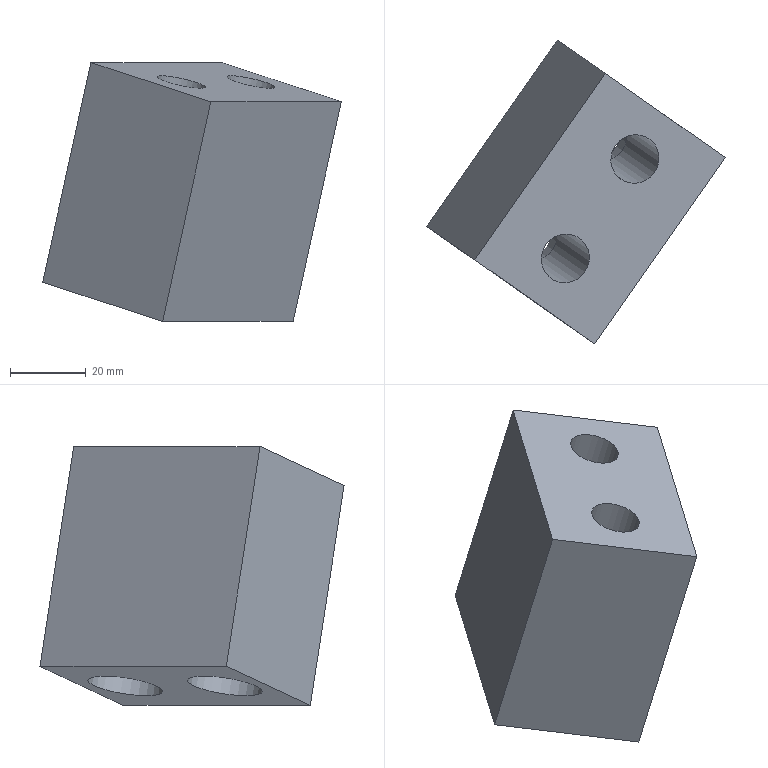Part | NX | features solid 2 | 1 solid | 12 faces | box 78.785 x 80.218 x 68.308 mm | volume 120815 mm3 | plane 8 | cylinder 4 | commonest cylinder face diameters 13 x2 20 x2
STEP:
#1=CARTESIAN_POINT('',(27.002,617.117,-490.837));
#2=VERTEX_POINT('',#1);
#3=CARTESIAN_POINT('',(21.858,620.718,-489.155));
#4=DIRECTION('',(-0.212,0.1485,-0.9659));
#5=DIRECTION('',(0.7912,-0.554,-0.2588));
#6=AXIS2_PLACEMENT_3D('',#3,#4,#5);
#7=CIRCLE('',#6,6.5);
#8=EDGE_CURVE('',#2,#2,#7,.F.);
#9=ORIENTED_EDGE('',*,*,#8,.F.);
#10=EDGE_LOOP('',(#9));
#11=FACE_BOUND('',#10,.T.);
#12=CARTESIAN_POINT('',(8.647,590.904,-490.837));
#13=VERTEX_POINT('',#12);
#14=CARTESIAN_POINT('',(3.504,594.505,-489.155));
#15=DIRECTION('',(-0.212,0.1485,-0.9659));
#16=DIRECTION('',(0.7912,-0.554,-0.2588));
#17=AXIS2_PLACEMENT_3D('',#14,#15,#16);
#18=CIRCLE('',#17,6.5);
#19=EDGE_CURVE('',#13,#13,#18,.F.);
#20=ORIENTED_EDGE('',*,*,#19,.F.);
#21=EDGE_LOOP('',(#20));
#22=FACE_BOUND('',#21,.T.);
#23=CARTESIAN_POINT('',(11.299,571.956,-494.331));
#24=VERTEX_POINT('',#23);
#25=CARTESIAN_POINT('',(-20.351,594.118,-483.978));
#26=VERTEX_POINT('',#25);
#27=CARTESIAN_POINT('',(11.299,571.956,-494.331));
#28=DIRECTION('',(0.7912,-0.554,-0.2588));
#29=VECTOR('',#28,1000.);
#30=LINE('',#27,#29);
#31=EDGE_CURVE('',#24,#26,#30,.F.);
#32=ORIENTED_EDGE('',*,*,#31,.F.);
#33=CARTESIAN_POINT('',(45.713,621.106,-494.331));
#34=VERTEX_POINT('',#33);
#35=CARTESIAN_POINT('',(45.713,621.106,-494.331));
#36=DIRECTION('',(-0.5736,-0.8192,0.));
#37=VECTOR('',#36,1000.);
#38=LINE('',#35,#37);
#39=EDGE_CURVE('',#34,#24,#38,.T.);
#40=ORIENTED_EDGE('',*,*,#39,.F.);
#41=CARTESIAN_POINT('',(14.064,643.267,-483.978));
#42=VERTEX_POINT('',#41);
#43=CARTESIAN_POINT('',(45.713,621.106,-494.331));
#44=DIRECTION('',(0.7912,-0.554,-0.2588));
#45=VECTOR('',#44,1000.);
#46=LINE('',#43,#45);
#47=EDGE_CURVE('',#34,#42,#46,.F.);
#48=ORIENTED_EDGE('',*,*,#47,.T.);
#49=CARTESIAN_POINT('',(14.064,643.267,-483.978));
#50=DIRECTION('',(-0.5736,-0.8192,0.));
#51=VECTOR('',#50,1000.);
#52=LINE('',#49,#51);
#53=EDGE_CURVE('',#42,#26,#52,.T.);
#54=ORIENTED_EDGE('',*,*,#53,.T.);
#55=EDGE_LOOP('',(#32,#40,#48,#54));
#56=FACE_BOUND('',#55,.T.);
#57=CARTESIAN_POINT('',(45.713,621.106,-494.331));
#58=DIRECTION('',(0.212,-0.1485,0.9659));
#59=DIRECTION('',(-0.5736,-0.8192,0.));
#60=AXIS2_PLACEMENT_3D('',#57,#58,#59);
#61=PLANE('',#60);
#62=ADVANCED_FACE('',(#11,#22,#56),#61,.T.);
#63=ORIENTED_EDGE('',*,*,#47,.F.);
#64=CARTESIAN_POINT('',(32.993,630.013,-552.287));
#65=VERTEX_POINT('',#64);
#66=CARTESIAN_POINT('',(45.713,621.106,-494.331));
#67=DIRECTION('',(-0.212,0.1485,-0.9659));
#68=VECTOR('',#67,1000.);
#69=LINE('',#66,#68);
#70=EDGE_CURVE('',#34,#65,#69,.T.);
#71=ORIENTED_EDGE('',*,*,#70,.T.);
#72=CARTESIAN_POINT('',(1.343,652.174,-541.934));
#73=VERTEX_POINT('',#72);
#74=CARTESIAN_POINT('',(32.993,630.013,-552.287));
#75=DIRECTION('',(-0.7912,0.554,0.2588));
#76=VECTOR('',#75,1000.);
#77=LINE('',#74,#76);
#78=EDGE_CURVE('',#65,#73,#77,.T.);
#79=ORIENTED_EDGE('',*,*,#78,.T.);
#80=CARTESIAN_POINT('',(14.064,643.267,-483.978));
#81=DIRECTION('',(0.212,-0.1485,0.9659));
#82=VECTOR('',#81,1000.);
#83=LINE('',#80,#82);
#84=EDGE_CURVE('',#42,#73,#83,.F.);
#85=ORIENTED_EDGE('',*,*,#84,.F.);
#86=EDGE_LOOP('',(#63,#71,#79,#85));
#87=FACE_BOUND('',#86,.T.);
#88=CARTESIAN_POINT('',(45.713,621.106,-494.331));
#89=DIRECTION('',(-0.5736,-0.8192,0.));
#90=DIRECTION('',(-0.212,0.1485,-0.9659));
#91=AXIS2_PLACEMENT_3D('',#88,#89,#90);
#92=PLANE('',#91);
#93=ADVANCED_FACE('',(#87),#92,.F.);
#94=CARTESIAN_POINT('',(17.05,624.085,-549.698));
#95=VERTEX_POINT('',#94);
#96=CARTESIAN_POINT('',(9.138,629.625,-547.11));
#97=DIRECTION('',(-0.212,0.1485,-0.9659));
#98=DIRECTION('',(0.7912,-0.554,-0.2588));
#99=AXIS2_PLACEMENT_3D('',#96,#97,#98);
#100=CIRCLE('',#99,10.);
#101=EDGE_CURVE('',#95,#95,#100,.T.);
#102=ORIENTED_EDGE('',*,*,#101,.F.);
#103=EDGE_LOOP('',(#102));
#104=FACE_BOUND('',#103,.T.);
#105=CARTESIAN_POINT('',(-1.304,597.872,-549.698));
#106=VERTEX_POINT('',#105);
#107=CARTESIAN_POINT('',(-9.217,603.412,-547.11));
#108=DIRECTION('',(-0.212,0.1485,-0.9659));
#109=DIRECTION('',(0.7912,-0.554,-0.2588));
#110=AXIS2_PLACEMENT_3D('',#107,#108,#109);
#111=CIRCLE('',#110,10.);
#112=EDGE_CURVE('',#106,#106,#111,.T.);
#113=ORIENTED_EDGE('',*,*,#112,.F.);
#114=EDGE_LOOP('',(#113));
#115=FACE_BOUND('',#114,.T.);
#116=ORIENTED_EDGE('',*,*,#78,.F.);
#117=CARTESIAN_POINT('',(-1.422,580.864,-552.287));
#118=VERTEX_POINT('',#117);
#119=CARTESIAN_POINT('',(32.993,630.013,-552.287));
#120=DIRECTION('',(-0.5736,-0.8192,0.));
#121=VECTOR('',#120,1000.);
#122=LINE('',#119,#121);
#123=EDGE_CURVE('',#65,#118,#122,.T.);
#124=ORIENTED_EDGE('',*,*,#123,.T.);
#125=CARTESIAN_POINT('',(-33.072,603.025,-541.934));
#126=VERTEX_POINT('',#125);
#127=CARTESIAN_POINT('',(-1.422,580.864,-552.287));
#128=DIRECTION('',(0.7912,-0.554,-0.2588));
#129=VECTOR('',#128,1000.);
#130=LINE('',#127,#129);
#131=EDGE_CURVE('',#118,#126,#130,.F.);
#132=ORIENTED_EDGE('',*,*,#131,.T.);
#133=CARTESIAN_POINT('',(1.343,652.174,-541.934));
#134=DIRECTION('',(-0.5736,-0.8192,0.));
#135=VECTOR('',#134,1000.);
#136=LINE('',#133,#135);
#137=EDGE_CURVE('',#73,#126,#136,.T.);
#138=ORIENTED_EDGE('',*,*,#137,.F.);
#139=EDGE_LOOP('',(#116,#124,#132,#138));
#140=FACE_BOUND('',#139,.T.);
#141=CARTESIAN_POINT('',(32.993,630.013,-552.287));
#142=DIRECTION('',(0.212,-0.1485,0.9659));
#143=DIRECTION('',(-0.5736,-0.8192,0.));
#144=AXIS2_PLACEMENT_3D('',#141,#142,#143);
#145=PLANE('',#144);
#146=ADVANCED_FACE('',(#104,#115,#140),#145,.F.);
#147=CARTESIAN_POINT('',(11.299,571.956,-494.331));
#148=DIRECTION('',(-0.212,0.1485,-0.9659));
#149=VECTOR('',#148,1000.);
#150=LINE('',#147,#149);
#151=EDGE_CURVE('',#24,#118,#150,.T.);
#152=ORIENTED_EDGE('',*,*,#151,.F.);
#153=ORIENTED_EDGE('',*,*,#31,.T.);
#154=CARTESIAN_POINT('',(-20.351,594.118,-483.978));
#155=DIRECTION('',(0.212,-0.1485,0.9659));
#156=VECTOR('',#155,1000.);
#157=LINE('',#154,#156);
#158=EDGE_CURVE('',#26,#126,#157,.F.);
#159=ORIENTED_EDGE('',*,*,#158,.T.);
#160=ORIENTED_EDGE('',*,*,#131,.F.);
#161=EDGE_LOOP('',(#152,#153,#159,#160));
#162=FACE_BOUND('',#161,.T.);
#163=CARTESIAN_POINT('',(11.299,571.956,-494.331));
#164=DIRECTION('',(-0.5736,-0.8192,0.));
#165=DIRECTION('',(-0.212,0.1485,-0.9659));
#166=AXIS2_PLACEMENT_3D('',#163,#164,#165);
#167=PLANE('',#166);
#168=ADVANCED_FACE('',(#162),#167,.T.);
#169=ORIENTED_EDGE('',*,*,#137,.T.);
#170=ORIENTED_EDGE('',*,*,#158,.F.);
#171=ORIENTED_EDGE('',*,*,#53,.F.);
#172=ORIENTED_EDGE('',*,*,#84,.T.);
#173=EDGE_LOOP('',(#169,#170,#171,#172));
#174=FACE_BOUND('',#173,.T.);
#175=CARTESIAN_POINT('',(14.064,643.267,-483.978));
#176=DIRECTION('',(-0.7912,0.554,0.2588));
#177=DIRECTION('',(0.212,-0.1485,0.9659));
#178=AXIS2_PLACEMENT_3D('',#175,#176,#177);
#179=PLANE('',#178);
#180=ADVANCED_FACE('',(#174),#179,.T.);
#181=ORIENTED_EDGE('',*,*,#123,.F.);
#182=ORIENTED_EDGE('',*,*,#70,.F.);
#183=ORIENTED_EDGE('',*,*,#39,.T.);
#184=ORIENTED_EDGE('',*,*,#151,.T.);
#185=EDGE_LOOP('',(#181,#182,#183,#184));
#186=FACE_BOUND('',#185,.T.);
#187=CARTESIAN_POINT('',(45.713,621.106,-494.331));
#188=DIRECTION('',(-0.7912,0.554,0.2588));
#189=DIRECTION('',(0.212,-0.1485,0.9659));
#190=AXIS2_PLACEMENT_3D('',#187,#188,#189);
#191=PLANE('',#190);
#192=ADVANCED_FACE('',(#186),#191,.F.);
#193=CARTESIAN_POINT('',(0.1666,596.842,-529.474));
#194=VERTEX_POINT('',#193);
#195=CARTESIAN_POINT('',(-4.976,600.443,-527.792));
#196=DIRECTION('',(-0.212,0.1485,-0.9659));
#197=DIRECTION('',(0.7912,-0.554,-0.2588));
#198=AXIS2_PLACEMENT_3D('',#195,#196,#197);
#199=CIRCLE('',#198,6.5);
#200=EDGE_CURVE('',#194,#194,#199,.T.);
#201=ORIENTED_EDGE('',*,*,#200,.T.);
#202=EDGE_LOOP('',(#201));
#203=FACE_BOUND('',#202,.T.);
#204=ORIENTED_EDGE('',*,*,#19,.T.);
#205=EDGE_LOOP('',(#204));
#206=FACE_BOUND('',#205,.T.);
#207=CARTESIAN_POINT('',(7.744,591.536,-469.836));
#208=DIRECTION('',(0.212,-0.1485,0.9659));
#209=DIRECTION('',(0.7912,-0.554,-0.2588));
#210=AXIS2_PLACEMENT_3D('',#207,#208,#209);
#211=CYLINDRICAL_SURFACE('',#210,6.5);
#212=ADVANCED_FACE('',(#203,#206),#211,.F.);
#213=ORIENTED_EDGE('',*,*,#200,.F.);
#214=EDGE_LOOP('',(#213));
#215=FACE_BOUND('',#214,.T.);
#216=CARTESIAN_POINT('',(2.936,594.903,-530.38));
#217=VERTEX_POINT('',#216);
#218=CARTESIAN_POINT('',(-4.976,600.443,-527.792));
#219=DIRECTION('',(-0.212,0.1485,-0.9659));
#220=DIRECTION('',(0.7912,-0.554,-0.2588));
#221=AXIS2_PLACEMENT_3D('',#218,#219,#220);
#222=CIRCLE('',#221,10.);
#223=EDGE_CURVE('',#217,#217,#222,.T.);
#224=ORIENTED_EDGE('',*,*,#223,.T.);
#225=EDGE_LOOP('',(#224));
#226=FACE_BOUND('',#225,.T.);
#227=CARTESIAN_POINT('',(-6.124,598.805,-527.792));
#228=DIRECTION('',(0.212,-0.1485,0.9659));
#229=DIRECTION('',(0.7912,-0.554,-0.2588));
#230=AXIS2_PLACEMENT_3D('',#227,#228,#229);
#231=PLANE('',#230);
#232=ADVANCED_FACE('',(#215,#226),#231,.F.);
#233=ORIENTED_EDGE('',*,*,#223,.F.);
#234=EDGE_LOOP('',(#233));
#235=FACE_BOUND('',#234,.T.);
#236=ORIENTED_EDGE('',*,*,#112,.T.);
#237=EDGE_LOOP('',(#236));
#238=FACE_BOUND('',#237,.T.);
#239=CARTESIAN_POINT('',(-9.217,603.412,-547.11));
#240=DIRECTION('',(0.212,-0.1485,0.9659));
#241=DIRECTION('',(0.7912,-0.554,-0.2588));
#242=AXIS2_PLACEMENT_3D('',#239,#240,#241);
#243=CYLINDRICAL_SURFACE('',#242,10.);
#244=ADVANCED_FACE('',(#235,#238),#243,.F.);
#245=CARTESIAN_POINT('',(18.521,623.055,-529.474));
#246=VERTEX_POINT('',#245);
#247=CARTESIAN_POINT('',(13.378,626.656,-527.792));
#248=DIRECTION('',(-0.212,0.1485,-0.9659));
#249=DIRECTION('',(0.7912,-0.554,-0.2588));
#250=AXIS2_PLACEMENT_3D('',#247,#248,#249);
#251=CIRCLE('',#250,6.5);
#252=EDGE_CURVE('',#246,#246,#251,.T.);
#253=ORIENTED_EDGE('',*,*,#252,.T.);
#254=EDGE_LOOP('',(#253));
#255=FACE_BOUND('',#254,.T.);
#256=ORIENTED_EDGE('',*,*,#8,.T.);
#257=EDGE_LOOP('',(#256));
#258=FACE_BOUND('',#257,.T.);
#259=CARTESIAN_POINT('',(26.099,617.749,-469.836));
#260=DIRECTION('',(0.212,-0.1485,0.9659));
#261=DIRECTION('',(0.7912,-0.554,-0.2588));
#262=AXIS2_PLACEMENT_3D('',#259,#260,#261);
#263=CYLINDRICAL_SURFACE('',#262,6.5);
#264=ADVANCED_FACE('',(#255,#258),#263,.F.);
#265=ORIENTED_EDGE('',*,*,#252,.F.);
#266=EDGE_LOOP('',(#265));
#267=FACE_BOUND('',#266,.T.);
#268=CARTESIAN_POINT('',(21.29,621.116,-530.38));
#269=VERTEX_POINT('',#268);
#270=CARTESIAN_POINT('',(13.378,626.656,-527.792));
#271=DIRECTION('',(-0.212,0.1485,-0.9659));
#272=DIRECTION('',(0.7912,-0.554,-0.2588));
#273=AXIS2_PLACEMENT_3D('',#270,#271,#272);
#274=CIRCLE('',#273,10.);
#275=EDGE_CURVE('',#269,#269,#274,.T.);
#276=ORIENTED_EDGE('',*,*,#275,.T.);
#277=EDGE_LOOP('',(#276));
#278=FACE_BOUND('',#277,.T.);
#279=CARTESIAN_POINT('',(14.525,628.294,-527.792));
#280=DIRECTION('',(0.212,-0.1485,0.9659));
#281=DIRECTION('',(0.7912,-0.554,-0.2588));
#282=AXIS2_PLACEMENT_3D('',#279,#280,#281);
#283=PLANE('',#282);
#284=ADVANCED_FACE('',(#267,#278),#283,.F.);
#285=ORIENTED_EDGE('',*,*,#275,.F.);
#286=EDGE_LOOP('',(#285));
#287=FACE_BOUND('',#286,.T.);
#288=ORIENTED_EDGE('',*,*,#101,.T.);
#289=EDGE_LOOP('',(#288));
#290=FACE_BOUND('',#289,.T.);
#291=CARTESIAN_POINT('',(9.138,629.625,-547.11));
#292=DIRECTION('',(0.212,-0.1485,0.9659));
#293=DIRECTION('',(0.7912,-0.554,-0.2588));
#294=AXIS2_PLACEMENT_3D('',#291,#292,#293);
#295=CYLINDRICAL_SURFACE('',#294,10.);
#296=ADVANCED_FACE('',(#287,#290),#295,.F.);
#297=CLOSED_SHELL('',(#62,#93,#146,#168,#180,#192,#212,#232,#244,#264,#284,#296));
#298=MANIFOLD_SOLID_BREP('',#297);
#299=(LENGTH_UNIT()NAMED_UNIT(*)SI_UNIT(.MILLI.,.METRE.));
#300=UNCERTAINTY_MEASURE_WITH_UNIT(LENGTH_MEASURE(0.00001),#299,'','');
#301=(NAMED_UNIT(*)PLANE_ANGLE_UNIT()SI_UNIT($,.RADIAN.));
#302=(NAMED_UNIT(*)SI_UNIT($,.STERADIAN.)SOLID_ANGLE_UNIT());
#303=(GEOMETRIC_REPRESENTATION_CONTEXT(3)GLOBAL_UNCERTAINTY_ASSIGNED_CONTEXT((#300))GLOBAL_UNIT_ASSIGNED_CONTEXT((#299,#301,#302))REPRESENTATION_CONTEXT('',''));
#304=ADVANCED_BREP_SHAPE_REPRESENTATION('',(#298),#303);